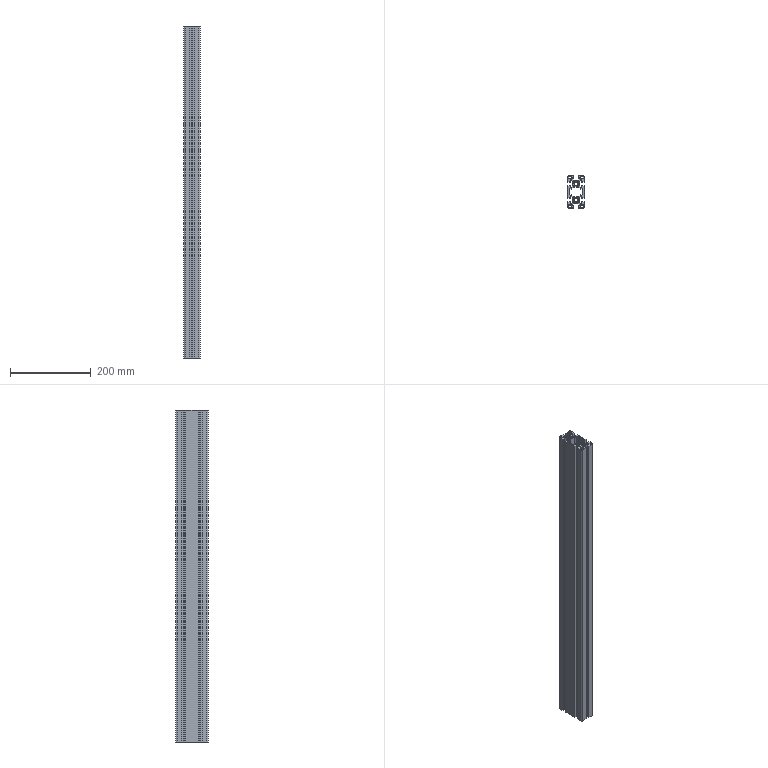Part | NX | features BREP 1 | 1 solid | 182 faces | box 40 x 80 x 820 mm | volume 913686 mm3 | plane 112 | cylinder 70 | commonest cylinder face diameters 2 x36 0.76 x20 10.5 x10 6 x4